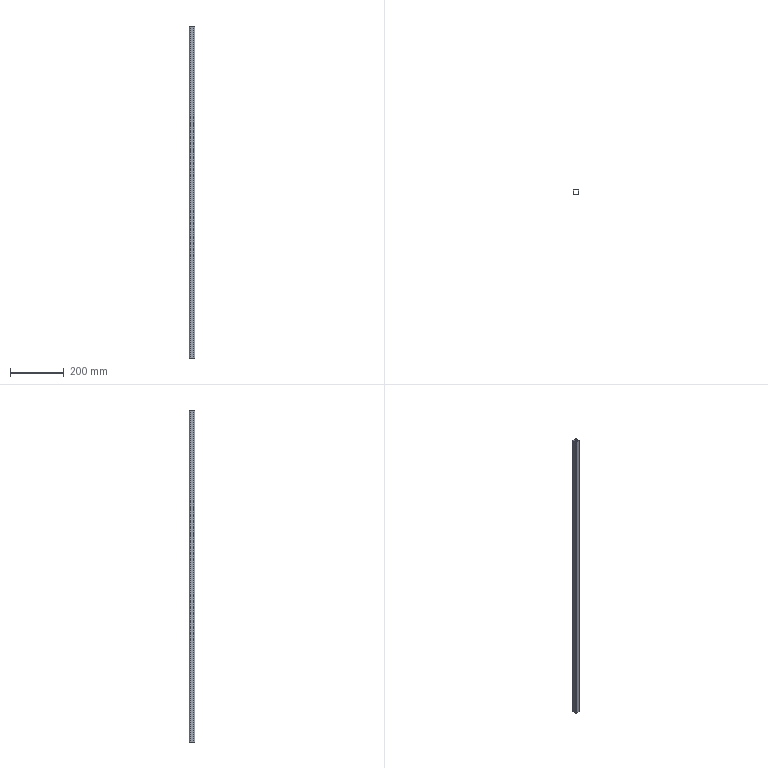Part | SolidWorks | features BaseBody 1 | 1 solid | 18 faces | box 20 x 20 x 1236 mm | volume 105425 mm3 | plane 10 | cylinder 8 | commonest cylinder face diameters 3.6 x4 6 x4
STEP:
#1=CARTESIAN_POINT('',(7.,-8.8,0.));
#2=VERTEX_POINT('',#1);
#3=CARTESIAN_POINT('',(7.,-8.8,1236.));
#4=VERTEX_POINT('',#3);
#5=CARTESIAN_POINT('',(7.,-8.8,0.));
#6=DIRECTION('',(0.,0.,1.));
#7=VECTOR('',#6,1000.);
#8=LINE('',#5,#7);
#9=EDGE_CURVE('',#2,#4,#8,.T.);
#10=ORIENTED_EDGE('',*,*,#9,.F.);
#11=CARTESIAN_POINT('',(-7.,-8.8,0.));
#12=VERTEX_POINT('',#11);
#13=CARTESIAN_POINT('',(7.,-8.8,0.));
#14=DIRECTION('',(1.,0.,0.));
#15=VECTOR('',#14,1000.);
#16=LINE('',#13,#15);
#17=EDGE_CURVE('',#12,#2,#16,.T.);
#18=ORIENTED_EDGE('',*,*,#17,.F.);
#19=CARTESIAN_POINT('',(-7.,-8.8,1236.));
#20=VERTEX_POINT('',#19);
#21=CARTESIAN_POINT('',(-7.,-8.8,0.));
#22=DIRECTION('',(0.,0.,-1.));
#23=VECTOR('',#22,1000.);
#24=LINE('',#21,#23);
#25=EDGE_CURVE('',#20,#12,#24,.T.);
#26=ORIENTED_EDGE('',*,*,#25,.F.);
#27=CARTESIAN_POINT('',(7.,-8.8,1236.));
#28=DIRECTION('',(-1.,0.,0.));
#29=VECTOR('',#28,1000.);
#30=LINE('',#27,#29);
#31=EDGE_CURVE('',#4,#20,#30,.T.);
#32=ORIENTED_EDGE('',*,*,#31,.F.);
#33=EDGE_LOOP('',(#10,#18,#26,#32));
#34=FACE_OUTER_BOUND('',#33,.T.);
#35=CARTESIAN_POINT('',(7.,-8.8,0.));
#36=DIRECTION('',(0.,-1.,0.));
#37=DIRECTION('',(1.,0.,0.));
#38=AXIS2_PLACEMENT_3D('',#35,#36,#37);
#39=PLANE('',#38);
#40=ADVANCED_FACE('',(#34),#39,.F.);
#41=CARTESIAN_POINT('',(-8.8,-7.,1236.));
#42=VERTEX_POINT('',#41);
#43=CARTESIAN_POINT('',(-8.8,7.,1236.));
#44=VERTEX_POINT('',#43);
#45=CARTESIAN_POINT('',(-8.8,0.,1236.));
#46=DIRECTION('',(0.,1.,0.));
#47=VECTOR('',#46,1000.);
#48=LINE('',#45,#47);
#49=EDGE_CURVE('',#42,#44,#48,.T.);
#50=ORIENTED_EDGE('',*,*,#49,.T.);
#51=CARTESIAN_POINT('',(-7.,8.8,1236.));
#52=VERTEX_POINT('',#51);
#53=CARTESIAN_POINT('',(-7.,7.,1236.));
#54=DIRECTION('',(0.,0.,-1.));
#55=DIRECTION('',(1.,0.,0.));
#56=AXIS2_PLACEMENT_3D('',#53,#54,#55);
#57=CIRCLE('',#56,1.8);
#58=EDGE_CURVE('',#44,#52,#57,.T.);
#59=ORIENTED_EDGE('',*,*,#58,.T.);
#60=CARTESIAN_POINT('',(7.,8.8,1236.));
#61=VERTEX_POINT('',#60);
#62=CARTESIAN_POINT('',(0.,8.8,1236.));
#63=DIRECTION('',(1.,0.,0.));
#64=VECTOR('',#63,1000.);
#65=LINE('',#62,#64);
#66=EDGE_CURVE('',#52,#61,#65,.T.);
#67=ORIENTED_EDGE('',*,*,#66,.T.);
#68=CARTESIAN_POINT('',(8.8,7.,1236.));
#69=VERTEX_POINT('',#68);
#70=CARTESIAN_POINT('',(7.,7.,1236.));
#71=DIRECTION('',(0.,0.,-1.));
#72=DIRECTION('',(1.,0.,0.));
#73=AXIS2_PLACEMENT_3D('',#70,#71,#72);
#74=CIRCLE('',#73,1.8);
#75=EDGE_CURVE('',#61,#69,#74,.T.);
#76=ORIENTED_EDGE('',*,*,#75,.T.);
#77=CARTESIAN_POINT('',(8.8,-7.,1236.));
#78=VERTEX_POINT('',#77);
#79=CARTESIAN_POINT('',(8.8,0.,1236.));
#80=DIRECTION('',(0.,-1.,0.));
#81=VECTOR('',#80,1000.);
#82=LINE('',#79,#81);
#83=EDGE_CURVE('',#69,#78,#82,.T.);
#84=ORIENTED_EDGE('',*,*,#83,.T.);
#85=CARTESIAN_POINT('',(7.,-7.,1236.));
#86=DIRECTION('',(0.,0.,-1.));
#87=DIRECTION('',(1.,0.,0.));
#88=AXIS2_PLACEMENT_3D('',#85,#86,#87);
#89=CIRCLE('',#88,1.8);
#90=EDGE_CURVE('',#78,#4,#89,.T.);
#91=ORIENTED_EDGE('',*,*,#90,.T.);
#92=ORIENTED_EDGE('',*,*,#31,.T.);
#93=CARTESIAN_POINT('',(-7.,-7.,1236.));
#94=DIRECTION('',(0.,0.,-1.));
#95=DIRECTION('',(1.,0.,0.));
#96=AXIS2_PLACEMENT_3D('',#93,#94,#95);
#97=CIRCLE('',#96,1.8);
#98=EDGE_CURVE('',#20,#42,#97,.T.);
#99=ORIENTED_EDGE('',*,*,#98,.T.);
#100=EDGE_LOOP('',(#50,#59,#67,#76,#84,#91,#92,#99));
#101=FACE_BOUND('',#100,.T.);
#102=CARTESIAN_POINT('',(7.,10.,1236.));
#103=VERTEX_POINT('',#102);
#104=CARTESIAN_POINT('',(-7.,10.,1236.));
#105=VERTEX_POINT('',#104);
#106=CARTESIAN_POINT('',(0.,10.,1236.));
#107=DIRECTION('',(-1.,0.,0.));
#108=VECTOR('',#107,1000.);
#109=LINE('',#106,#108);
#110=EDGE_CURVE('',#103,#105,#109,.T.);
#111=ORIENTED_EDGE('',*,*,#110,.T.);
#112=CARTESIAN_POINT('',(-10.,7.,1236.));
#113=VERTEX_POINT('',#112);
#114=CARTESIAN_POINT('',(-7.,7.,1236.));
#115=DIRECTION('',(0.,0.,1.));
#116=DIRECTION('',(1.,0.,0.));
#117=AXIS2_PLACEMENT_3D('',#114,#115,#116);
#118=CIRCLE('',#117,3.);
#119=EDGE_CURVE('',#105,#113,#118,.T.);
#120=ORIENTED_EDGE('',*,*,#119,.T.);
#121=CARTESIAN_POINT('',(-10.,-7.,1236.));
#122=VERTEX_POINT('',#121);
#123=CARTESIAN_POINT('',(-10.,0.,1236.));
#124=DIRECTION('',(0.,-1.,0.));
#125=VECTOR('',#124,1000.);
#126=LINE('',#123,#125);
#127=EDGE_CURVE('',#113,#122,#126,.T.);
#128=ORIENTED_EDGE('',*,*,#127,.T.);
#129=CARTESIAN_POINT('',(-7.,-10.,1236.));
#130=VERTEX_POINT('',#129);
#131=CARTESIAN_POINT('',(-7.,-7.,1236.));
#132=DIRECTION('',(0.,0.,1.));
#133=DIRECTION('',(1.,0.,0.));
#134=AXIS2_PLACEMENT_3D('',#131,#132,#133);
#135=CIRCLE('',#134,3.);
#136=EDGE_CURVE('',#122,#130,#135,.T.);
#137=ORIENTED_EDGE('',*,*,#136,.T.);
#138=CARTESIAN_POINT('',(7.,-10.,1236.));
#139=VERTEX_POINT('',#138);
#140=CARTESIAN_POINT('',(0.,-10.,1236.));
#141=DIRECTION('',(1.,0.,0.));
#142=VECTOR('',#141,1000.);
#143=LINE('',#140,#142);
#144=EDGE_CURVE('',#130,#139,#143,.T.);
#145=ORIENTED_EDGE('',*,*,#144,.T.);
#146=CARTESIAN_POINT('',(10.,-7.,1236.));
#147=VERTEX_POINT('',#146);
#148=CARTESIAN_POINT('',(7.,-7.,1236.));
#149=DIRECTION('',(0.,0.,1.));
#150=DIRECTION('',(1.,0.,0.));
#151=AXIS2_PLACEMENT_3D('',#148,#149,#150);
#152=CIRCLE('',#151,3.);
#153=EDGE_CURVE('',#139,#147,#152,.T.);
#154=ORIENTED_EDGE('',*,*,#153,.T.);
#155=CARTESIAN_POINT('',(10.,7.,1236.));
#156=VERTEX_POINT('',#155);
#157=CARTESIAN_POINT('',(10.,0.,1236.));
#158=DIRECTION('',(0.,1.,0.));
#159=VECTOR('',#158,1000.);
#160=LINE('',#157,#159);
#161=EDGE_CURVE('',#147,#156,#160,.T.);
#162=ORIENTED_EDGE('',*,*,#161,.T.);
#163=CARTESIAN_POINT('',(7.,7.,1236.));
#164=DIRECTION('',(0.,0.,1.));
#165=DIRECTION('',(1.,0.,0.));
#166=AXIS2_PLACEMENT_3D('',#163,#164,#165);
#167=CIRCLE('',#166,3.);
#168=EDGE_CURVE('',#156,#103,#167,.T.);
#169=ORIENTED_EDGE('',*,*,#168,.T.);
#170=EDGE_LOOP('',(#111,#120,#128,#137,#145,#154,#162,#169));
#171=FACE_OUTER_BOUND('',#170,.T.);
#172=CARTESIAN_POINT('',(0.,0.,1236.));
#173=DIRECTION('',(0.,0.,1.));
#174=DIRECTION('',(1.,0.,0.));
#175=AXIS2_PLACEMENT_3D('',#172,#173,#174);
#176=PLANE('',#175);
#177=ADVANCED_FACE('',(#101,#171),#176,.T.);
#178=CARTESIAN_POINT('',(8.8,-7.,0.));
#179=VERTEX_POINT('',#178);
#180=CARTESIAN_POINT('',(8.8,-7.,0.));
#181=DIRECTION('',(0.,0.,1.));
#182=VECTOR('',#181,1000.);
#183=LINE('',#180,#182);
#184=EDGE_CURVE('',#179,#78,#183,.T.);
#185=ORIENTED_EDGE('',*,*,#184,.F.);
#186=CARTESIAN_POINT('',(7.,-7.,0.));
#187=DIRECTION('',(0.,0.,1.));
#188=DIRECTION('',(1.,0.,0.));
#189=AXIS2_PLACEMENT_3D('',#186,#187,#188);
#190=CIRCLE('',#189,1.8);
#191=EDGE_CURVE('',#2,#179,#190,.T.);
#192=ORIENTED_EDGE('',*,*,#191,.F.);
#193=ORIENTED_EDGE('',*,*,#9,.T.);
#194=ORIENTED_EDGE('',*,*,#90,.F.);
#195=EDGE_LOOP('',(#185,#192,#193,#194));
#196=FACE_OUTER_BOUND('',#195,.T.);
#197=CARTESIAN_POINT('',(7.,-7.,0.));
#198=DIRECTION('',(0.,0.,1.));
#199=DIRECTION('',(1.,0.,0.));
#200=AXIS2_PLACEMENT_3D('',#197,#198,#199);
#201=CYLINDRICAL_SURFACE('',#200,1.8);
#202=ADVANCED_FACE('',(#196),#201,.F.);
#203=CARTESIAN_POINT('',(-8.8,7.,0.));
#204=VERTEX_POINT('',#203);
#205=CARTESIAN_POINT('',(-7.,8.8,0.));
#206=VERTEX_POINT('',#205);
#207=CARTESIAN_POINT('',(-7.,7.,0.));
#208=DIRECTION('',(0.,0.,-1.));
#209=DIRECTION('',(1.,0.,0.));
#210=AXIS2_PLACEMENT_3D('',#207,#208,#209);
#211=CIRCLE('',#210,1.8);
#212=EDGE_CURVE('',#204,#206,#211,.T.);
#213=ORIENTED_EDGE('',*,*,#212,.F.);
#214=CARTESIAN_POINT('',(-8.8,-7.,0.));
#215=VERTEX_POINT('',#214);
#216=CARTESIAN_POINT('',(-8.8,0.,0.));
#217=DIRECTION('',(0.,1.,0.));
#218=VECTOR('',#217,1000.);
#219=LINE('',#216,#218);
#220=EDGE_CURVE('',#215,#204,#219,.T.);
#221=ORIENTED_EDGE('',*,*,#220,.F.);
#222=CARTESIAN_POINT('',(-7.,-7.,0.));
#223=DIRECTION('',(0.,0.,-1.));
#224=DIRECTION('',(1.,0.,0.));
#225=AXIS2_PLACEMENT_3D('',#222,#223,#224);
#226=CIRCLE('',#225,1.8);
#227=EDGE_CURVE('',#12,#215,#226,.T.);
#228=ORIENTED_EDGE('',*,*,#227,.F.);
#229=ORIENTED_EDGE('',*,*,#17,.T.);
#230=ORIENTED_EDGE('',*,*,#191,.T.);
#231=CARTESIAN_POINT('',(8.8,7.,0.));
#232=VERTEX_POINT('',#231);
#233=CARTESIAN_POINT('',(8.8,0.,0.));
#234=DIRECTION('',(0.,-1.,0.));
#235=VECTOR('',#234,1000.);
#236=LINE('',#233,#235);
#237=EDGE_CURVE('',#232,#179,#236,.T.);
#238=ORIENTED_EDGE('',*,*,#237,.F.);
#239=CARTESIAN_POINT('',(7.,8.8,0.));
#240=VERTEX_POINT('',#239);
#241=CARTESIAN_POINT('',(7.,7.,0.));
#242=DIRECTION('',(0.,0.,-1.));
#243=DIRECTION('',(1.,0.,0.));
#244=AXIS2_PLACEMENT_3D('',#241,#242,#243);
#245=CIRCLE('',#244,1.8);
#246=EDGE_CURVE('',#240,#232,#245,.T.);
#247=ORIENTED_EDGE('',*,*,#246,.F.);
#248=CARTESIAN_POINT('',(0.,8.8,0.));
#249=DIRECTION('',(1.,0.,0.));
#250=VECTOR('',#249,1000.);
#251=LINE('',#248,#250);
#252=EDGE_CURVE('',#206,#240,#251,.T.);
#253=ORIENTED_EDGE('',*,*,#252,.F.);
#254=EDGE_LOOP('',(#213,#221,#228,#229,#230,#238,#247,#253));
#255=FACE_BOUND('',#254,.T.);
#256=CARTESIAN_POINT('',(-7.,10.,0.));
#257=VERTEX_POINT('',#256);
#258=CARTESIAN_POINT('',(-10.,7.,0.));
#259=VERTEX_POINT('',#258);
#260=CARTESIAN_POINT('',(-7.,7.,0.));
#261=DIRECTION('',(0.,0.,1.));
#262=DIRECTION('',(1.,0.,0.));
#263=AXIS2_PLACEMENT_3D('',#260,#261,#262);
#264=CIRCLE('',#263,3.);
#265=EDGE_CURVE('',#257,#259,#264,.T.);
#266=ORIENTED_EDGE('',*,*,#265,.F.);
#267=CARTESIAN_POINT('',(7.,10.,0.));
#268=VERTEX_POINT('',#267);
#269=CARTESIAN_POINT('',(0.,10.,0.));
#270=DIRECTION('',(-1.,0.,0.));
#271=VECTOR('',#270,1000.);
#272=LINE('',#269,#271);
#273=EDGE_CURVE('',#268,#257,#272,.T.);
#274=ORIENTED_EDGE('',*,*,#273,.F.);
#275=CARTESIAN_POINT('',(10.,7.,0.));
#276=VERTEX_POINT('',#275);
#277=CARTESIAN_POINT('',(7.,7.,0.));
#278=DIRECTION('',(0.,0.,1.));
#279=DIRECTION('',(1.,0.,0.));
#280=AXIS2_PLACEMENT_3D('',#277,#278,#279);
#281=CIRCLE('',#280,3.);
#282=EDGE_CURVE('',#276,#268,#281,.T.);
#283=ORIENTED_EDGE('',*,*,#282,.F.);
#284=CARTESIAN_POINT('',(10.,-7.,0.));
#285=VERTEX_POINT('',#284);
#286=CARTESIAN_POINT('',(10.,0.,0.));
#287=DIRECTION('',(0.,1.,0.));
#288=VECTOR('',#287,1000.);
#289=LINE('',#286,#288);
#290=EDGE_CURVE('',#285,#276,#289,.T.);
#291=ORIENTED_EDGE('',*,*,#290,.F.);
#292=CARTESIAN_POINT('',(7.,-10.,0.));
#293=VERTEX_POINT('',#292);
#294=CARTESIAN_POINT('',(7.,-7.,0.));
#295=DIRECTION('',(0.,0.,1.));
#296=DIRECTION('',(1.,0.,0.));
#297=AXIS2_PLACEMENT_3D('',#294,#295,#296);
#298=CIRCLE('',#297,3.);
#299=EDGE_CURVE('',#293,#285,#298,.T.);
#300=ORIENTED_EDGE('',*,*,#299,.F.);
#301=CARTESIAN_POINT('',(-7.,-10.,0.));
#302=VERTEX_POINT('',#301);
#303=CARTESIAN_POINT('',(0.,-10.,0.));
#304=DIRECTION('',(1.,0.,0.));
#305=VECTOR('',#304,1000.);
#306=LINE('',#303,#305);
#307=EDGE_CURVE('',#302,#293,#306,.T.);
#308=ORIENTED_EDGE('',*,*,#307,.F.);
#309=CARTESIAN_POINT('',(-10.,-7.,0.));
#310=VERTEX_POINT('',#309);
#311=CARTESIAN_POINT('',(-7.,-7.,0.));
#312=DIRECTION('',(0.,0.,1.));
#313=DIRECTION('',(1.,0.,0.));
#314=AXIS2_PLACEMENT_3D('',#311,#312,#313);
#315=CIRCLE('',#314,3.);
#316=EDGE_CURVE('',#310,#302,#315,.T.);
#317=ORIENTED_EDGE('',*,*,#316,.F.);
#318=CARTESIAN_POINT('',(-10.,0.,0.));
#319=DIRECTION('',(0.,-1.,0.));
#320=VECTOR('',#319,1000.);
#321=LINE('',#318,#320);
#322=EDGE_CURVE('',#259,#310,#321,.T.);
#323=ORIENTED_EDGE('',*,*,#322,.F.);
#324=EDGE_LOOP('',(#266,#274,#283,#291,#300,#308,#317,#323));
#325=FACE_OUTER_BOUND('',#324,.T.);
#326=CARTESIAN_POINT('',(0.,0.,0.));
#327=DIRECTION('',(0.,0.,1.));
#328=DIRECTION('',(1.,0.,0.));
#329=AXIS2_PLACEMENT_3D('',#326,#327,#328);
#330=PLANE('',#329);
#331=ADVANCED_FACE('',(#255,#325),#330,.F.);
#332=ORIENTED_EDGE('',*,*,#25,.T.);
#333=ORIENTED_EDGE('',*,*,#227,.T.);
#334=CARTESIAN_POINT('',(-8.8,-7.,0.));
#335=DIRECTION('',(0.,0.,-1.));
#336=VECTOR('',#335,1000.);
#337=LINE('',#334,#336);
#338=EDGE_CURVE('',#42,#215,#337,.T.);
#339=ORIENTED_EDGE('',*,*,#338,.F.);
#340=ORIENTED_EDGE('',*,*,#98,.F.);
#341=EDGE_LOOP('',(#332,#333,#339,#340));
#342=FACE_OUTER_BOUND('',#341,.T.);
#343=CARTESIAN_POINT('',(-7.,-7.,0.));
#344=DIRECTION('',(0.,0.,1.));
#345=DIRECTION('',(1.,0.,0.));
#346=AXIS2_PLACEMENT_3D('',#343,#344,#345);
#347=CYLINDRICAL_SURFACE('',#346,1.8);
#348=ADVANCED_FACE('',(#342),#347,.F.);
#349=CARTESIAN_POINT('',(-8.8,7.,0.));
#350=DIRECTION('',(0.,0.,1.));
#351=VECTOR('',#350,1000.);
#352=LINE('',#349,#351);
#353=EDGE_CURVE('',#204,#44,#352,.T.);
#354=ORIENTED_EDGE('',*,*,#353,.F.);
#355=ORIENTED_EDGE('',*,*,#212,.T.);
#356=CARTESIAN_POINT('',(-7.,8.8,0.));
#357=DIRECTION('',(0.,0.,-1.));
#358=VECTOR('',#357,1000.);
#359=LINE('',#356,#358);
#360=EDGE_CURVE('',#52,#206,#359,.T.);
#361=ORIENTED_EDGE('',*,*,#360,.F.);
#362=ORIENTED_EDGE('',*,*,#58,.F.);
#363=EDGE_LOOP('',(#354,#355,#361,#362));
#364=FACE_OUTER_BOUND('',#363,.T.);
#365=CARTESIAN_POINT('',(-7.,7.,0.));
#366=DIRECTION('',(0.,0.,1.));
#367=DIRECTION('',(1.,0.,0.));
#368=AXIS2_PLACEMENT_3D('',#365,#366,#367);
#369=CYLINDRICAL_SURFACE('',#368,1.8);
#370=ADVANCED_FACE('',(#364),#369,.F.);
#371=ORIENTED_EDGE('',*,*,#338,.T.);
#372=ORIENTED_EDGE('',*,*,#220,.T.);
#373=ORIENTED_EDGE('',*,*,#353,.T.);
#374=ORIENTED_EDGE('',*,*,#49,.F.);
#375=EDGE_LOOP('',(#371,#372,#373,#374));
#376=FACE_OUTER_BOUND('',#375,.T.);
#377=CARTESIAN_POINT('',(-8.8,-7.,0.));
#378=DIRECTION('',(-1.,0.,0.));
#379=DIRECTION('',(0.,-1.,0.));
#380=AXIS2_PLACEMENT_3D('',#377,#378,#379);
#381=PLANE('',#380);
#382=ADVANCED_FACE('',(#376),#381,.F.);
#383=CARTESIAN_POINT('',(8.8,7.,0.));
#384=DIRECTION('',(0.,0.,1.));
#385=VECTOR('',#384,1000.);
#386=LINE('',#383,#385);
#387=EDGE_CURVE('',#232,#69,#386,.T.);
#388=ORIENTED_EDGE('',*,*,#387,.F.);
#389=ORIENTED_EDGE('',*,*,#237,.T.);
#390=ORIENTED_EDGE('',*,*,#184,.T.);
#391=ORIENTED_EDGE('',*,*,#83,.F.);
#392=EDGE_LOOP('',(#388,#389,#390,#391));
#393=FACE_OUTER_BOUND('',#392,.T.);
#394=CARTESIAN_POINT('',(8.8,7.,0.));
#395=DIRECTION('',(1.,0.,0.));
#396=DIRECTION('',(0.,0.,-1.));
#397=AXIS2_PLACEMENT_3D('',#394,#395,#396);
#398=PLANE('',#397);
#399=ADVANCED_FACE('',(#393),#398,.F.);
#400=CARTESIAN_POINT('',(7.,8.8,0.));
#401=DIRECTION('',(0.,0.,1.));
#402=VECTOR('',#401,1000.);
#403=LINE('',#400,#402);
#404=EDGE_CURVE('',#240,#61,#403,.T.);
#405=ORIENTED_EDGE('',*,*,#404,.F.);
#406=ORIENTED_EDGE('',*,*,#246,.T.);
#407=ORIENTED_EDGE('',*,*,#387,.T.);
#408=ORIENTED_EDGE('',*,*,#75,.F.);
#409=EDGE_LOOP('',(#405,#406,#407,#408));
#410=FACE_OUTER_BOUND('',#409,.T.);
#411=CARTESIAN_POINT('',(7.,7.,0.));
#412=DIRECTION('',(0.,0.,1.));
#413=DIRECTION('',(1.,0.,0.));
#414=AXIS2_PLACEMENT_3D('',#411,#412,#413);
#415=CYLINDRICAL_SURFACE('',#414,1.8);
#416=ADVANCED_FACE('',(#410),#415,.F.);
#417=ORIENTED_EDGE('',*,*,#360,.T.);
#418=ORIENTED_EDGE('',*,*,#252,.T.);
#419=ORIENTED_EDGE('',*,*,#404,.T.);
#420=ORIENTED_EDGE('',*,*,#66,.F.);
#421=EDGE_LOOP('',(#417,#418,#419,#420));
#422=FACE_OUTER_BOUND('',#421,.T.);
#423=CARTESIAN_POINT('',(-7.,8.8,0.));
#424=DIRECTION('',(0.,1.,0.));
#425=DIRECTION('',(-1.,0.,0.));
#426=AXIS2_PLACEMENT_3D('',#423,#424,#425);
#427=PLANE('',#426);
#428=ADVANCED_FACE('',(#422),#427,.F.);
#429=ORIENTED_EDGE('',*,*,#265,.T.);
#430=CARTESIAN_POINT('',(-10.,7.,0.));
#431=DIRECTION('',(0.,0.,1.));
#432=VECTOR('',#431,1000.);
#433=LINE('',#430,#432);
#434=EDGE_CURVE('',#259,#113,#433,.T.);
#435=ORIENTED_EDGE('',*,*,#434,.T.);
#436=ORIENTED_EDGE('',*,*,#119,.F.);
#437=CARTESIAN_POINT('',(-7.,10.,0.));
#438=DIRECTION('',(0.,0.,-1.));
#439=VECTOR('',#438,1000.);
#440=LINE('',#437,#439);
#441=EDGE_CURVE('',#105,#257,#440,.T.);
#442=ORIENTED_EDGE('',*,*,#441,.T.);
#443=EDGE_LOOP('',(#429,#435,#436,#442));
#444=FACE_OUTER_BOUND('',#443,.T.);
#445=CARTESIAN_POINT('',(-7.,7.,0.));
#446=DIRECTION('',(0.,0.,1.));
#447=DIRECTION('',(1.,0.,0.));
#448=AXIS2_PLACEMENT_3D('',#445,#446,#447);
#449=CYLINDRICAL_SURFACE('',#448,3.);
#450=ADVANCED_FACE('',(#444),#449,.T.);
#451=ORIENTED_EDGE('',*,*,#273,.T.);
#452=ORIENTED_EDGE('',*,*,#441,.F.);
#453=ORIENTED_EDGE('',*,*,#110,.F.);
#454=CARTESIAN_POINT('',(7.,10.,0.));
#455=DIRECTION('',(0.,0.,-1.));
#456=VECTOR('',#455,1000.);
#457=LINE('',#454,#456);
#458=EDGE_CURVE('',#103,#268,#457,.T.);
#459=ORIENTED_EDGE('',*,*,#458,.T.);
#460=EDGE_LOOP('',(#451,#452,#453,#459));
#461=FACE_OUTER_BOUND('',#460,.T.);
#462=CARTESIAN_POINT('',(-7.,10.,0.));
#463=DIRECTION('',(0.,1.,0.));
#464=DIRECTION('',(-1.,0.,0.));
#465=AXIS2_PLACEMENT_3D('',#462,#463,#464);
#466=PLANE('',#465);
#467=ADVANCED_FACE('',(#461),#466,.T.);
#468=ORIENTED_EDGE('',*,*,#282,.T.);
#469=ORIENTED_EDGE('',*,*,#458,.F.);
#470=ORIENTED_EDGE('',*,*,#168,.F.);
#471=CARTESIAN_POINT('',(10.,7.,0.));
#472=DIRECTION('',(0.,0.,-1.));
#473=VECTOR('',#472,1000.);
#474=LINE('',#471,#473);
#475=EDGE_CURVE('',#156,#276,#474,.T.);
#476=ORIENTED_EDGE('',*,*,#475,.T.);
#477=EDGE_LOOP('',(#468,#469,#470,#476));
#478=FACE_OUTER_BOUND('',#477,.T.);
#479=CARTESIAN_POINT('',(7.,7.,0.));
#480=DIRECTION('',(0.,0.,1.));
#481=DIRECTION('',(1.,0.,0.));
#482=AXIS2_PLACEMENT_3D('',#479,#480,#481);
#483=CYLINDRICAL_SURFACE('',#482,3.);
#484=ADVANCED_FACE('',(#478),#483,.T.);
#485=ORIENTED_EDGE('',*,*,#290,.T.);
#486=ORIENTED_EDGE('',*,*,#475,.F.);
#487=ORIENTED_EDGE('',*,*,#161,.F.);
#488=CARTESIAN_POINT('',(10.,-7.,0.));
#489=DIRECTION('',(0.,0.,-1.));
#490=VECTOR('',#489,1000.);
#491=LINE('',#488,#490);
#492=EDGE_CURVE('',#147,#285,#491,.T.);
#493=ORIENTED_EDGE('',*,*,#492,.T.);
#494=EDGE_LOOP('',(#485,#486,#487,#493));
#495=FACE_OUTER_BOUND('',#494,.T.);
#496=CARTESIAN_POINT('',(10.,7.,0.));
#497=DIRECTION('',(1.,0.,0.));
#498=DIRECTION('',(0.,0.,-1.));
#499=AXIS2_PLACEMENT_3D('',#496,#497,#498);
#500=PLANE('',#499);
#501=ADVANCED_FACE('',(#495),#500,.T.);
#502=ORIENTED_EDGE('',*,*,#299,.T.);
#503=ORIENTED_EDGE('',*,*,#492,.F.);
#504=ORIENTED_EDGE('',*,*,#153,.F.);
#505=CARTESIAN_POINT('',(7.,-10.,0.));
#506=DIRECTION('',(0.,0.,-1.));
#507=VECTOR('',#506,1000.);
#508=LINE('',#505,#507);
#509=EDGE_CURVE('',#139,#293,#508,.T.);
#510=ORIENTED_EDGE('',*,*,#509,.T.);
#511=EDGE_LOOP('',(#502,#503,#504,#510));
#512=FACE_OUTER_BOUND('',#511,.T.);
#513=CARTESIAN_POINT('',(7.,-7.,0.));
#514=DIRECTION('',(0.,0.,1.));
#515=DIRECTION('',(1.,0.,0.));
#516=AXIS2_PLACEMENT_3D('',#513,#514,#515);
#517=CYLINDRICAL_SURFACE('',#516,3.);
#518=ADVANCED_FACE('',(#512),#517,.T.);
#519=ORIENTED_EDGE('',*,*,#307,.T.);
#520=ORIENTED_EDGE('',*,*,#509,.F.);
#521=ORIENTED_EDGE('',*,*,#144,.F.);
#522=CARTESIAN_POINT('',(-7.,-10.,0.));
#523=DIRECTION('',(0.,0.,-1.));
#524=VECTOR('',#523,1000.);
#525=LINE('',#522,#524);
#526=EDGE_CURVE('',#130,#302,#525,.T.);
#527=ORIENTED_EDGE('',*,*,#526,.T.);
#528=EDGE_LOOP('',(#519,#520,#521,#527));
#529=FACE_OUTER_BOUND('',#528,.T.);
#530=CARTESIAN_POINT('',(7.,-10.,0.));
#531=DIRECTION('',(0.,-1.,0.));
#532=DIRECTION('',(1.,0.,0.));
#533=AXIS2_PLACEMENT_3D('',#530,#531,#532);
#534=PLANE('',#533);
#535=ADVANCED_FACE('',(#529),#534,.T.);
#536=ORIENTED_EDGE('',*,*,#316,.T.);
#537=ORIENTED_EDGE('',*,*,#526,.F.);
#538=ORIENTED_EDGE('',*,*,#136,.F.);
#539=CARTESIAN_POINT('',(-10.,-7.,0.));
#540=DIRECTION('',(0.,0.,-1.));
#541=VECTOR('',#540,1000.);
#542=LINE('',#539,#541);
#543=EDGE_CURVE('',#122,#310,#542,.T.);
#544=ORIENTED_EDGE('',*,*,#543,.T.);
#545=EDGE_LOOP('',(#536,#537,#538,#544));
#546=FACE_OUTER_BOUND('',#545,.T.);
#547=CARTESIAN_POINT('',(-7.,-7.,0.));
#548=DIRECTION('',(0.,0.,1.));
#549=DIRECTION('',(1.,0.,0.));
#550=AXIS2_PLACEMENT_3D('',#547,#548,#549);
#551=CYLINDRICAL_SURFACE('',#550,3.);
#552=ADVANCED_FACE('',(#546),#551,.T.);
#553=ORIENTED_EDGE('',*,*,#322,.T.);
#554=ORIENTED_EDGE('',*,*,#543,.F.);
#555=ORIENTED_EDGE('',*,*,#127,.F.);
#556=ORIENTED_EDGE('',*,*,#434,.F.);
#557=EDGE_LOOP('',(#553,#554,#555,#556));
#558=FACE_OUTER_BOUND('',#557,.T.);
#559=CARTESIAN_POINT('',(-10.,-7.,0.));
#560=DIRECTION('',(-1.,0.,0.));
#561=DIRECTION('',(0.,-1.,0.));
#562=AXIS2_PLACEMENT_3D('',#559,#560,#561);
#563=PLANE('',#562);
#564=ADVANCED_FACE('',(#558),#563,.T.);
#565=CLOSED_SHELL('',(#40,#177,#202,#331,#348,#370,#382,#399,#416,#428,#450,#467,#484,#501,#518,#535,#552,#564));
#566=MANIFOLD_SOLID_BREP('',#565);
#567=CARTESIAN_POINT('',(0.,0.,0.));
#568=DIRECTION('',(0.,0.,1.));
#569=DIRECTION('',(1.,0.,0.));
#570=AXIS2_PLACEMENT_3D('',#567,#568,#569);
#571=(LENGTH_UNIT()NAMED_UNIT(*)SI_UNIT(.MILLI.,.METRE.));
#572=UNCERTAINTY_MEASURE_WITH_UNIT(LENGTH_MEASURE(0.00001),#571,'','');
#573=(NAMED_UNIT(*)PLANE_ANGLE_UNIT()SI_UNIT($,.RADIAN.));
#574=(NAMED_UNIT(*)SI_UNIT($,.STERADIAN.)SOLID_ANGLE_UNIT());
#575=(GEOMETRIC_REPRESENTATION_CONTEXT(3)GLOBAL_UNCERTAINTY_ASSIGNED_CONTEXT((#572))GLOBAL_UNIT_ASSIGNED_CONTEXT((#571,#573,#574))REPRESENTATION_CONTEXT('',''));
#576=ADVANCED_BREP_SHAPE_REPRESENTATION('',(#566,#570),#575);